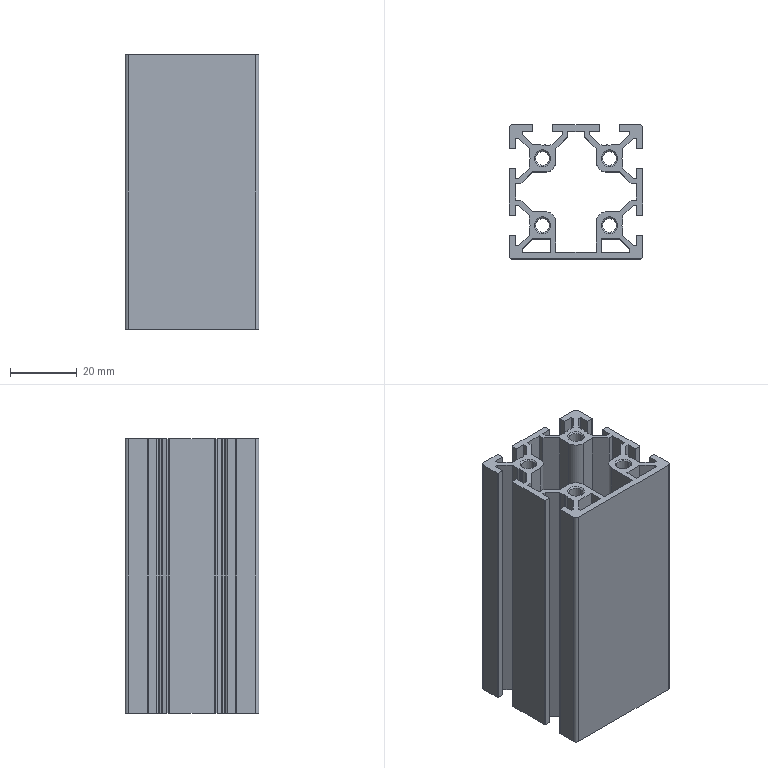Part | STEP file | 0245_025_HFSF5-4040-82-LTP | 1 solid | 174 faces | box 40 x 40 x 82 mm | volume 42687 mm3 | plane 130 | cylinder 36 | cone 8 | commonest cylinder face diameters 0.6 x12 1 x8 4.2 x8 2 x4 6 x4